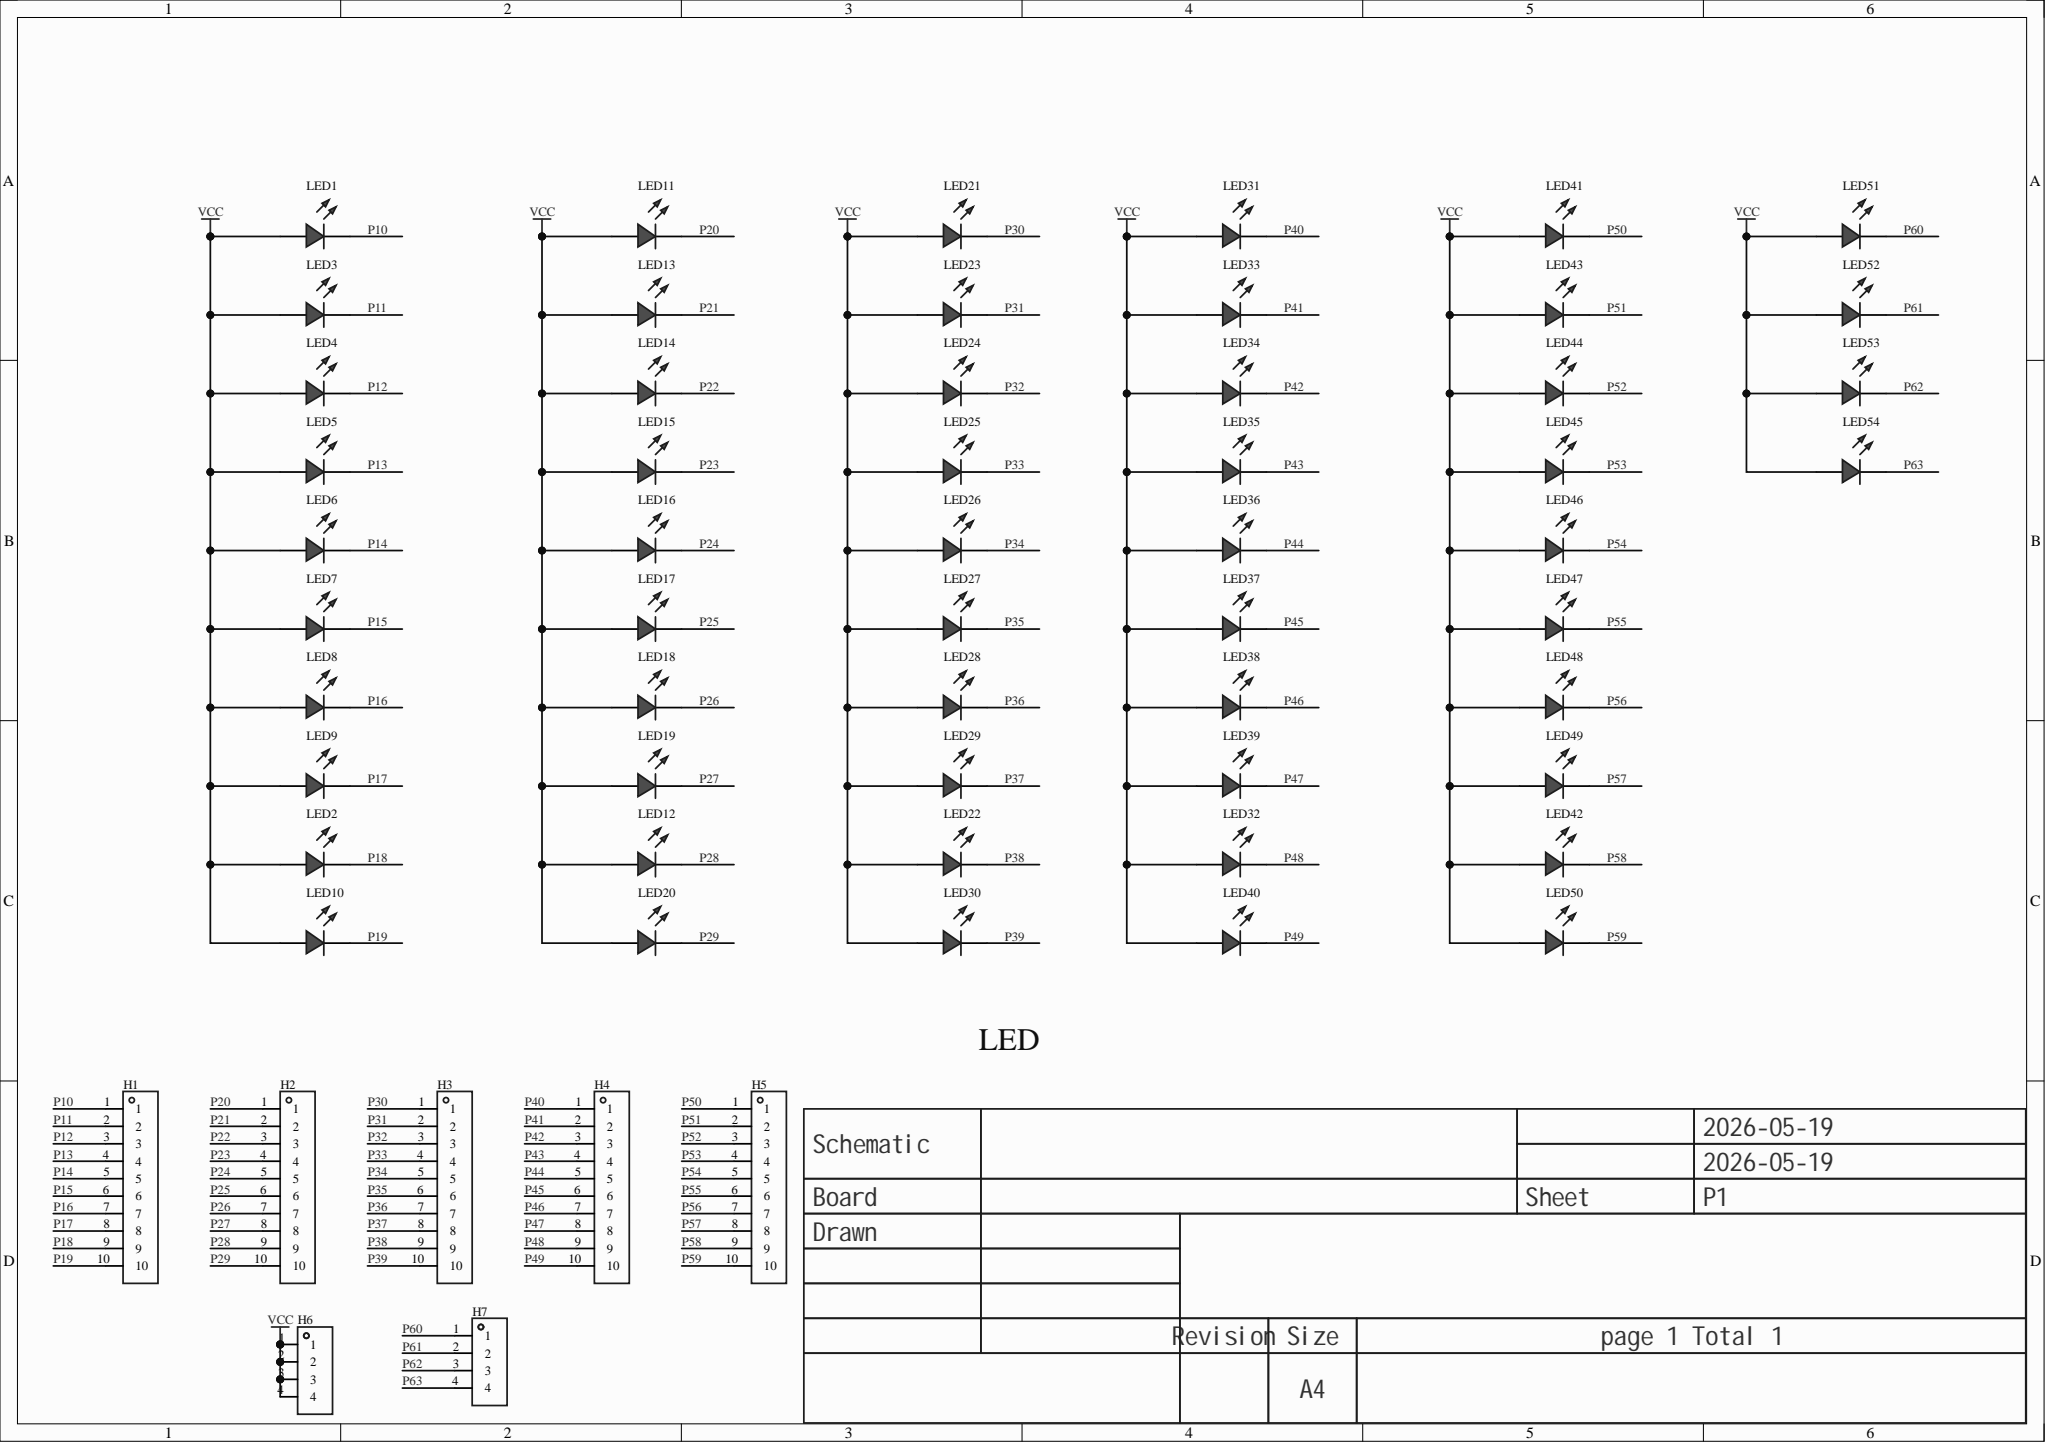Circuit board | Altium Designer | 61 parts | 55 nets
Bill of materials:
Comment,Description,Designator,Footprint,LibRef,Quantity
"","","H1, H2, H3, H4, H5","HDR-TH_10P-P2.54-V-F","HDR-F_2.54_1x10P","5"
"","","H6, H7","HDR-TH_4P-P2.54-V-F","HDR-F_2.54_1x4P","2"
"","","LED1, LED2, LED3, LED4, LED5, LED6, LED7, LED8, LED9, LED10, LED11, LED12, LED13, LED14, LED15, LED16, LED17, LED18, LED19, LED20, LED21, LED22, LED23, LED24, LED25, LED26, LED27, LED28, LED29, LED30, LED31, LED32, LED33, LED34, LED35, LED36, LED37, LED38, LED39, LED40, LED41, LED42, LED43, LED44, LED45, LED46, LED47, LED48, LED49, LED50, LED51, LED52, LED53, LED54","LED_TH-3mm","LED_TH-R_3mm","54"
Netlist (Protel format):
[
H1
HDR-TH_10P-P2.54-V-F




]
[
H2
HDR-TH_10P-P2.54-V-F




]
[
H3
HDR-TH_10P-P2.54-V-F




]
[
H4
HDR-TH_10P-P2.54-V-F




]
[
H5
HDR-TH_10P-P2.54-V-F




]
[
H6
HDR-TH_4P-P2.54-V-F




]
[
H7
HDR-TH_4P-P2.54-V-F




]
[
LED1
LED_TH-3mm




]
[
LED2
LED_TH-3mm




]
[
LED3
LED_TH-3mm




]
[
LED4
LED_TH-3mm




]
[
LED5
LED_TH-3mm




]
[
LED6
LED_TH-3mm




]
[
LED7
LED_TH-3mm




]
[
LED8
LED_TH-3mm




]
[
LED9
LED_TH-3mm




]
[
LED10
LED_TH-3mm




]
[
LED11
LED_TH-3mm




]
[
LED12
LED_TH-3mm




]
[
LED13
LED_TH-3mm




]
[
LED14
LED_TH-3mm




]
[
LED15
LED_TH-3mm




]
[
LED16
LED_TH-3mm




]
[
LED17
LED_TH-3mm




]
[
LED18
LED_TH-3mm




]
[
LED19
LED_TH-3mm




]
[
LED20
LED_TH-3mm




]
[
LED21
LED_TH-3mm




]
[
LED22
LED_TH-3mm




]
[
LED23
LED_TH-3mm




]
[
LED24
LED_TH-3mm




]
[
LED25
LED_TH-3mm




]
[
LED26
LED_TH-3mm




]
[
LED27
LED_TH-3mm




]
[
LED28
LED_TH-3mm




]
[
LED29
LED_TH-3mm




]
[
LED30
LED_TH-3mm




]
[
LED31
LED_TH-3mm




]
[
LED32
LED_TH-3mm




]
[
LED33
LED_TH-3mm




]
[
LED34
LED_TH-3mm




]
[
LED35
LED_TH-3mm




]
[
LED36
LED_TH-3mm




]
[
LED37
LED_TH-3mm




]
[
LED38
LED_TH-3mm




]
[
LED39
LED_TH-3mm




]
[
LED40
LED_TH-3mm




]
[
LED41
LED_TH-3mm




]
[
LED42
LED_TH-3mm




]
[
LED43
LED_TH-3mm




]
[
LED44
LED_TH-3mm




]
[
LED45
LED_TH-3mm




]
[
LED46
LED_TH-3mm




]
[
LED47
LED_TH-3mm




]
[
LED48
LED_TH-3mm




]
[
LED49
LED_TH-3mm




]
[
LED50
LED_TH-3mm




]
[
LED51
LED_TH-3mm




]
[
LED52
LED_TH-3mm




]
[
LED53
LED_TH-3mm




]
[
LED54
LED_TH-3mm




]
(
VCC
H6-1
H6-2
H6-3
H6-4
LED1-1
LED2-1
LED3-1
LED4-1
LED5-1
LED6-1
LED7-1
LED8-1
LED9-1
LED10-1
LED11-1
LED12-1
LED13-1
LED14-1
LED15-1
LED16-1
LED17-1
LED18-1
LED19-1
LED20-1
LED21-1
LED22-1
LED23-1
LED24-1
LED25-1
LED26-1
LED27-1
LED28-1
LED29-1
LED30-1
LED31-1
LED32-1
LED33-1
LED34-1
LED35-1
LED36-1
LED37-1
LED38-1
LED39-1
LED40-1
LED41-1
LED42-1
LED43-1
LED44-1
LED45-1
LED46-1
LED47-1
LED48-1
LED49-1
LED50-1
LED51-1
LED52-1
LED53-1
LED54-1
)
(
P63
H7-4
LED54-2
)
(
P62
H7-3
LED53-2
)
(
P61
H7-2
LED52-2
)
(
P60
H7-1
LED51-2
)
(
P59
H5-10
LED50-2
)
(
P58
H5-9
LED42-2
)
(
P57
H5-8
LED49-2
)
(
P56
H5-7
LED48-2
)
(
P55
H5-6
LED47-2
)
(
P54
H5-5
LED46-2
)
(
P53
H5-4
LED45-2
)
(
P52
H5-3
LED44-2
)
(
P51
H5-2
LED43-2
)
(
P50
H5-1
LED41-2
)
(
P49
H4-10
LED40-2
)
(
P48
H4-9
LED32-2
)
(
P47
H4-8
LED39-2
)
(
P46
H4-7
LED38-2
)
(
P45
H4-6
LED37-2
)
(
P44
H4-5
LED36-2
)
(
P43
H4-4
LED35-2
)
(
P42
H4-3
LED34-2
)
(
P41
H4-2
LED33-2
)
(
P40
H4-1
LED31-2
)
(
P39
H3-10
LED30-2
)
(
P38
H3-9
LED22-2
)
(
P37
H3-8
LED29-2
)
(
P36
H3-7
LED28-2
)
(
P35
H3-6
LED27-2
)
(
P34
H3-5
LED26-2
)
(
P33
H3-4
LED25-2
)
(
P32
H3-3
LED24-2
)
(
P31
H3-2
LED23-2
)
(
P30
H3-1
LED21-2
)
(
P29
H2-10
LED20-2
)
(
P28
H2-9
LED12-2
)
(
P27
H2-8
LED19-2
)
(
P26
H2-7
LED18-2
)
(
P25
H2-6
LED17-2
)
(
P24
H2-5
LED16-2
)
(
P23
H2-4
LED15-2
)
(
P22
H2-3
LED14-2
)
(
P21
H2-2
LED13-2
)
(
P20
H2-1
LED11-2
)
(
P19
H1-10
LED10-2
)
(
P18
H1-9
LED2-2
)
(
P17
H1-8
LED9-2
)
(
P16
H1-7
LED8-2
)
(
P15
H1-6
LED7-2
)
(
P14
H1-5
LED6-2
)
(
P13
H1-4
LED5-2
)
(
P12
H1-3
LED4-2
)
(
P11
H1-2
LED3-2
)
(
P10
H1-1
LED1-2
)